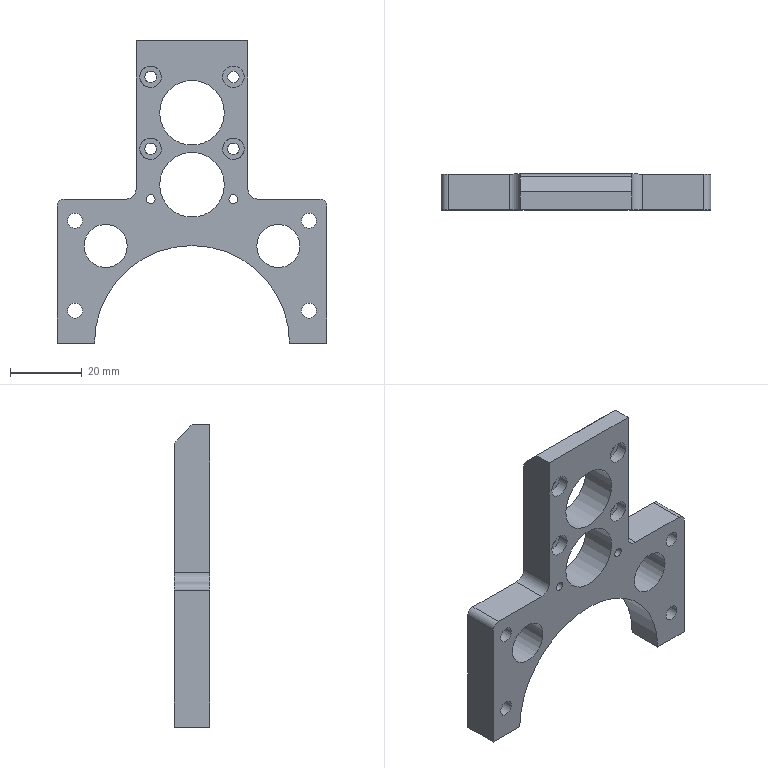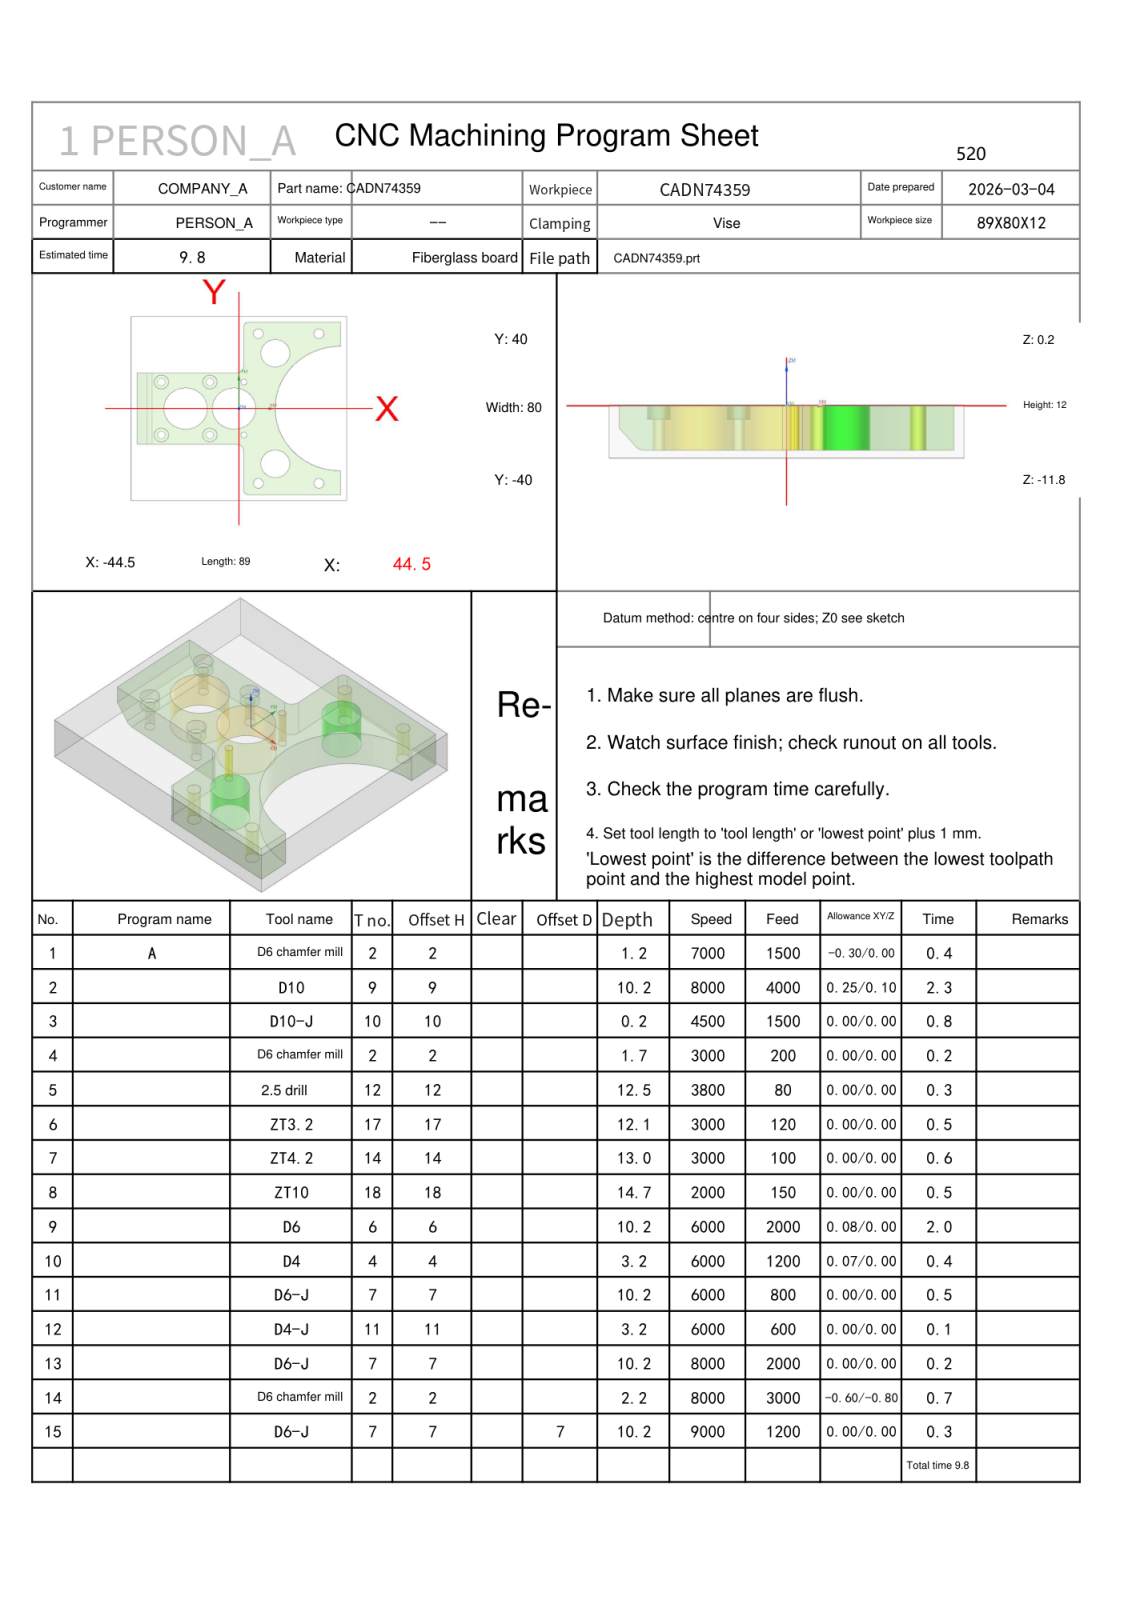NC program | NX | posted by the shop | part box 75 x 10 x 84 mm
Lines 168 to 1025 of 4435:
N2 T09 M06
(D10  D=10. R=0. H=09 ce=0.25 di=0.10)
G00 G90 G54 X55.978 Y-25.62 M03 S8000
G43 H09 Z50.
M08
Z-8.
G01 X55.879 Y-25.636 Z-8.625 F4000.
X55.78 Y-25.652 Z-8.872
X55.682 Y-25.668 Z-9.054
X55.583 Y-25.685 Z-9.2
X55.484 Y-25.701 Z-9.323
X55.386 Y-25.717 Z-9.428
X55.287 Y-25.733 Z-9.52
X55.188 Y-25.749 Z-9.6
X55.089 Y-25.765 Z-9.67
X54.991 Y-25.781 Z-9.732
X54.892 Y-25.798 Z-9.786
X54.793 Y-25.814 Z-9.833
X54.695 Y-25.83 Z-9.874
X54.596 Y-25.846 Z-9.908
X54.497 Y-25.862 Z-9.936
X54.399 Y-25.878 Z-9.96
X54.3 Y-25.894 Z-9.977
X54.201 Y-25.911 Z-9.99
X54.103 Y-25.927 Z-9.997
X54.004 Y-25.943 Z-10.
X51.921 Y-26.284
G03 X51.529 Y-26.606 I.085 J-.503
X51.003 Y-30.391 I13.335 J-3.785
G01 Y-30.428
G03 X50.867 Y-38.753 I808.367 J-17.329
G02 X45.986 Y-45.264 I-7.17 J.29
X39.917 Y-46.285 I-6.261 J18.659
X30.341 Y-46.411 I-9.576 J365.692
X27.499 Y-46.4 I0.0 J365.817
G01 X-42.921 Y-46.382
X-42.933
G02 X-49.794 Y-41.406 I0.0 J7.218
X-50.789 Y-35.332 I19.113 J6.252
X-50.91 Y-25.845 I373.69 J9.487
X-50.9 Y-23.093 I373.811 J0.0
G01 X-50.884 Y38.387
Y38.422
G02 X-45.84 Y45.328 I7.25 J0.0
X-39.701 Y46.297 I6.254 J-19.678
X-30.37 Y46.406 I9.331 J-401.405
X-28.122 Y46.4 I0.0 J-401.514
G01 X42.898 Y46.383
X42.927 Y46.384
G02 X49.811 Y41.386 I0.0 J-7.239
X50.775 Y35.669 I-18.441 J-6.051
X50.912 Y26.372 I-315.381 J-9.297
X50.9 Y23.55 I-315.518 J0.0
G01 X50.877 Y-24.489
G03 X50.286 Y-37.047 I142.408 J-13.003
G02 X45.587 Y-44.06 I-7.974 J.261
X39.258 Y-45.566 I-7.148 J15.994
X30.674 Y-45.811 I-8.584 J150.167
X28.643 Y-45.797 I0.0 J150.412
G01 X-41.507 Y-45.774
G02 X-48.576 Y-41.047 I.213 J7.967
X-50.058 Y-34.839 I15.926 J7.084
X-50.309 Y-26.406 I141.524 J8.433
X-50.297 Y-24.524 I141.775 J0.0
G01 X-50.275 Y36.987
G02 X-45.542 Y44.086 I7.968 J-.186
X-39.152 Y45.576 I7.153 J-16.226
X-30.828 Y45.807 I8.324 J-149.829
X-29.077 Y45.797 I0.0 J-150.06
G01 X41.427 Y45.778
G02 X48.594 Y41.026 I-.134 J-7.982
X50.058 Y34.865 I-15.941 J-7.044
X50.309 Y26.443 I-141.134 J-8.422
X50.297 Y24.551 I-141.385 J0.0
G01 X50.276 Y-23.129
G03 X49.777 Y-33.028 I390.595 J-24.675
G02 X49.784 Y-33.583 I-22.706 J-.555
X49.485 Y-37.255 I-22.713 J0.0
X44.185 Y-43.462 I-8.743 J2.1
X37.719 Y-44.938 I-7.537 J18.117
X28.329 Y-45.215 I-9.389 J158.915
X25.965 Y-45.197 I0.0 J159.192
G01 X-39.955 Y-45.175
G02 X-47.814 Y-39.98 I.188 J8.826
X-49.429 Y-33.31 I17.184 J7.691
X-49.71 Y-24.335 I143.051 J8.974
X-49.696 Y-22.336 I143.332 J0.0
G01 X-49.679 Y35.364
G02 X-44.459 Y43.33 I8.83 J-.092
X-38.022 Y44.911 I7.578 J-16.958
X-28.912 Y45.212 I9.111 J-137.745
X-26.809 Y45.196 I0.0 J-138.046
G01 X39.83 Y45.181
G02 X47.839 Y39.941 I-.065 J-8.84
X49.44 Y33.206 I-17.447 J-7.704
X49.714 Y23.912 I-157.529 J-9.293
X49.697 Y21.632 I-157.803 J0.0
G01 X49.678 Y-21.968
X49.225 Y-31.803
G02 X49.229 Y-32.188 I-20.81 J-.386
X48.802 Y-36.383 I-20.814 J0.0
X45.712 Y-41.212 I-8.978 J2.34
X41.095 Y-43.537 I-7.252 J8.659
X33.371 Y-44.494 I-8.027 J33.122
X22.83 Y-44.603 I-10.541 J509.682
X20.712 Y-44.599 I0.0 J509.791
G01 X-38.488 Y-44.575
G02 X-47.197 Y-38.782 I.085 J9.571
X-48.815 Y-31.864 I18.826 J8.052
X-49.109 Y-22.501 I149.03 J9.363
X-49.095 Y-20.47 I149.324 J0.0
G01 X-49.077 Y33.929
G02 X-43.199 Y42.74 I9.589 J-.031
X-36.212 Y44.33 I8.057 J-19.267
X-26.915 Y44.608 I9.297 J-155.073
X-24.938 Y44.596 I0.0 J-155.351
G01 X38.462 Y44.576
G02 X45.712 Y41.212 I-.038 J-9.578
X47.987 Y36.772 I-8.524 J-7.17
X48.987 Y29.054 I-31.871 J-8.053
X49.103 Y18.823 I-453.561 J-10.231
X49.098 Y16.875 I-453.677 J0.0
G01 X49.081 Y-20.845
G02 X48.512 Y-33.56 I-412.871 J12.098
X47.212 Y-37.787 I-11.192 J1.129
G01 X47.071 Y-38.859
X46.547 Y-40.125
X45.712 Y-41.212
X44.625 Y-42.047
X43.359 Y-42.571
G02 X36.862 Y-43.608 I-18.744 J96.529
X26.221 Y-44.01 I-10.642 J140.772
X24.093 Y-43.994 I0.0 J141.174
G01 X-37.027 Y-43.976
X-37.14 Y-43.977
G02 X-44.43 Y-40.927 I0.0 J10.236
X-47.637 Y-34.44 I9.99 J8.975
X-48.434 Y-25.973 I44.56 J8.467
G01 Y-25.851
G02 X-48.502 Y-16.338 I668.609 J9.513
X-48.498 Y-14.151 I668.677 J0.0
G01 X-48.477 Y32.509
X-48.478 Y32.633
G02 X-45.618 Y39.748 I10.279 J0.0
X-39.076 Y43.109 I9.049 J-9.568
X-30.73 Y43.925 I8.364 J-42.415
X-20.67 Y44.001 I10.06 J-670.02
X-18.79 Y43.998 I0.0 J-670.095
G01 X36.99 Y43.978
G02 X42.15 Y42.73 I-.05 J-11.506
G01 X43.359 Y42.571
X44.625 Y42.047
X45.672 Y41.243
X44.625 Y42.047
X43.359 Y42.571
X38.927 Y43.246
G03 X32.176 Y43.528 I-6.751 J-80.501
X30.655 Y43.514 I0.0 J-80.783
G01 X-27.705 Y43.49
G03 X-28.368 Y43.494 I-.663 J-67.088
X-36.921 Y42.946 I0.0 J-67.091
X-43.506 Y40.512 I1.842 J-15.105
X-47.595 Y33.6 I6.069 J-8.256
X-48.009 Y27.355 I46.897 J-6.245
X-48.002 Y26.539 I47.311 J0.0
G01 X-47.996 Y-22.581
G03 X-48.002 Y-23.52 I71.557 J-.939
X-47.457 Y-32.338 I71.563 J0.0
X-45.059 Y-38.933 I15.291 J1.827
X-38.134 Y-43.088 I8.297 J5.98
X-31.856 Y-43.51 I6.278 J46.515
X-31.013 Y-43.502 I0.0 J46.937
G01 X27.467 Y-43.496
G03 X28.363 Y-43.501 I.897 J84.045
X38.243 Y-42.918 I0.0 J84.049
G01 X39.379 Y-42.75
X41.998
X43.01 Y-42.617
X41.998 Y-42.75
G03 X39.64 Y-42.745 I-2.358 J-552.508
X26.893 Y-42.892 I0.0 J-552.513
G01 X-30.987 Y-42.896
G02 X-31.694 Y-42.903 I-.707 J36.738
X-37.738 Y-42.402 I0.0 J36.745
X-45.639 Y-35.699 I2.086 J10.465
X-47.152 Y-28.384 I22.469 J8.463
X-47.421 Y-19.046 I162.115 J9.338
X-47.415 Y-17.71 I162.384 J0.0
G01 X-47.39 Y26.97
G02 X-47.394 Y27.517 I33.144 J.547
X-46.865 Y33.418 I33.149 J0.0
X-40.255 Y41.119 I10.407 J-2.246
X-32.762 Y42.662 I8.552 J-22.554
X-22.513 Y42.931 I10.25 J-195.098
X-20.047 Y42.916 I0.0 J-195.367
G01 X32.913 Y42.895
G02 X37.059 Y42.75 I-3.312 J-153.901
G01 X42.002
X4.001
G02 X-1.94 Y42.44 I-5.941 J56.745
X-2.948 Y42.449 I0.0 J57.055
G01 X-26.644 Y42.398
G03 X-27.162 Y42.401 I-.518 J-58.199
X-35.911 Y41.739 I0.0 J-58.202
X-42.35 Y39.095 I2.145 J-14.385
X-46.294 Y32.394 I7.049 J-8.66
X-46.907 Y25.431 I39.25 J-6.963
X-46.904 Y24.93 I39.863 J0.0
G01 X-46.964 Y17.118
X-47.071 Y16.859
X-47.25 Y15.502
Y-15.498
G02 X-46.946 Y-20.425 I-41.193 J-5.017
G01 Y-20.474
G03 X-46.475 Y-29.878 I94.099 J0.0
X-44.401 Y-36.66 I17.549 J1.657
X-37.082 Y-41.751 I9.348 J5.635
X-30.309 Y-42.394 I6.773 J35.353
G01 X-30.043 Y-42.393
X-20.803 Y-42.437
X2.063 Y-42.455
X2.387 Y-42.568
X3.999 Y-42.75
X34.179
G02 X34.679 Y-43.25 I0.0 J-.5
X34.447 Y-43.672 I-.5 J0.0
G01 X33.688 Y-44.154
X32.018 Y-45.216 Z-9.9
X31.686 Y-45.427
X31.625 Y-45.46
X31.56 Y-45.484
X31.493 Y-45.499
X31.424 Y-45.505
X4.011 Y-45.829
X3.927 Y-45.823
X3.845 Y-45.802
X3.768 Y-45.769
X3.697 Y-45.723
X3.635 Y-45.666
X3.584 Y-45.599
X3.545 Y-45.524
X3.405 Y-45.195
X2.631 Y-43.374 Z-10.
X2.319 Y-42.658
G03 X1.312 Y-42.24 I-1.103 J-1.237
X-3.973 Y-41.861 I-5.285 J-36.647
X-4.603 Y-41.866 I0.0 J-37.027
G01 X-28.949 Y-41.801
G02 X-29.41 Y-41.804 I-.461 J37.313
X-36.23 Y-41.176 I0.0 J37.315
X-44.694 Y-33.743 I2.238 J11.085
X-46.111 Y-26.101 I25.417 J8.665
G01 X-46.444 Y-18.331
X-47.071 Y-16.859
X-47.142 Y-16.323
X-47.071 Y-16.859
G02 X-46.288 Y-18.758 I-19.509 J-9.157
X-45.837 Y-22.708 I-25.147 J-4.869
G03 X-45.021 Y-30.447 I53.163 J1.699
X-41.905 Y-37.052 I13.689 J2.42
X-35.072 Y-40.683 I8.907 J8.516
X-27.688 Y-41.32 I7.384 J42.526
X-27.309 Y-41.318 I0.0 J43.162
G01 X-4.438 Y-41.397
X-4.27
G02 X.312 Y-41.701 I0.0 J-34.683
G03 X1.817 Y-42.369 I2.752 J4.172
G02 X.115 Y-41.59 I1.508 J5.543
G03 X-3.709 Y-40.929 I-4.076 J-12.18
X-11.989 Y-40.751 I-8.28 J-193.082
X-13.61 Y-40.758 I0.0 J-193.26
G02 X-17.984 Y-40.779 I-4.374 J460.512
X-29.468 Y-40.635 I0.0 J460.533
X-36.376 Y-39.534 I.356 J24.457
X-43.581 Y-32.282 I3.881 J11.062
X-45.006 Y-25.185 I25.784 J8.869
G03 X-45.613 Y-19.657 I-53.321 J-3.05
G01 X-45.772 Y-19.135
X-46.539 Y-18.135
G02 X-45.484 Y-19.685 I-4.89 J-4.462
X-44.673 Y-24.041 I-19.233 J-5.834
G03 X-43.366 Y-31.047 I34.292 J2.772
X-34.429 Y-39.344 I11.592 J3.524
X-26.626 Y-40.207 I7.803 J34.842
G01 X-26.573
G03 X-13.716 Y-40.3 I12.857 J895.985
X-9.973 Y-40.292 I0.0 J896.077
G02 X-8.974 Y-40.284 I.999 J-61.074
X-2.064 Y-40.676 I0.0 J-61.082
X-.642 Y-41.046 I-.299 J-4.06
G03 X.293 Y-41.679 I3.825 J4.643
G02 X-.995 Y-40.8 I12.01 J18.986
G03 X-4.697 Y-39.958 I-4.256 J-10.154
X-13.146 Y-39.669 I-8.449 J-123.288
X-14.816 Y-39.681 I0.0 J-123.577
G02 X-17.977 Y-39.698 I-3.161 J282.289
X-28.411 Y-39.505 I0.0 J282.307
X-35.405 Y-38.215 I.667 J23.218
X-42.507 Y-30.802 I4.436 J11.359
X-43.957 Y-24.497 I29.071 J10.002
G03 X-44.861 Y-20.178 I-22.179 J-2.388
X-45.148 Y-19.645 I-2.368 J-.934
G01 X-45.712 Y-19.212
G02 X-44.343 Y-21.085 I-1.61 J-2.614
X-43.218 Y-26.093 I-38.835 J-11.359
G03 X-40.843 Y-32.734 I19.336 J3.169
X-33.229 Y-38.154 I10.555 J6.769
X-25.263 Y-39.109 I8.099 J33.868
X-10.491 Y-39.236 I15.426 J931.048
G02 X-10.043 Y-39.234 I.448 J-44.89
X-3.185 Y-39.761 I0.0 J-44.892
X-1.326 Y-40.363 I-1.209 J-6.911
G01 X-.647 Y-41.042
G03 X-3.589 Y-39.339 I-3.76 J-3.104
X-10.409 Y-38.673 I-6.821 J-34.624
G01 X-10.487 Y-38.674
X-24.004 Y-38.529
X-24.089
G02 X-32.162 Y-37.667 I0.0 J38.205
X-41.471 Y-29.37 I2.825 J12.541
X-43.15 Y-23.285 I46.847 J16.199
G03 X-44.329 Y-20.212 I-9.432 J-1.856
G02 X-45.101 Y-19.681 I4.994 J8.092
G03 X-44.363 Y-20.162 I1.751 J1.884
G02 X-43.084 Y-22.413 I-3.959 J-3.739
G01 X-41.479 Y-27.725
G03 X-37.233 Y-34.324 I13.721 J4.164
X-29.923 Y-37.464 I9.491 J12.016
X-21.493 Y-38.085 I8.43 J56.981
X-21.014 Y-38.083 I0.0 J57.601
G02 X-20.057 Y-38.081 I.957 J-307.575
X-8.281 Y-38.307 I0.0 J-307.576
X-2.849 Y-39.198 I-.51 J-20.109
X-1.851 Y-39.73 I-.792 J-2.69
G03 X-1.371 Y-40.317 I2.227 J1.328
G02 X-2.031 Y-39.512 I5.118 J4.867
G03 X-5.065 Y-38.243 I-4.075 J-5.479
X-12.566 Y-37.588 I-7.501 J-42.596
G01 X-12.576
G02 X-24.863 Y-37.347 I2.732 J452.627
X-32.465 Y-36.04 I.691 J26.789
X-40.216 Y-28.664 I4.515 J12.505
X-42.261 Y-23.056 I71.553 J29.275
G03 X-43.664 Y-20.469 I-7.417 J-2.347
G01 X-44.43 Y-20.128
G02 X-42.7 Y-21.538 I-.732 J-2.664
X-40.912 Y-25.618 I-21.873 J-12.018
G03 X-37.636 Y-31.607 I18.541 J6.251
X-29.785 Y-36.108 I10.661 J9.499
X-21.143 Y-36.969 I8.645 J42.957
G02 X-9.56 Y-37.254 I-2.044 J-318.823
X-3.802 Y-38.22 I-.712 J-21.872
X-2.276 Y-39.053 I-1.478 J-4.525
G01 X-1.861 Y-39.713
G03 X-4.109 Y-37.8 I-3.368 J-1.68
X-9.824 Y-36.714 I-6.597 J-19.142
X-21.242 Y-36.355 I-13.931 J-261.093
G02 X-29.456 Y-35.443 I.259 J39.8
X-39.091 Y-27.812 I3.147 J13.871
X-41.427 Y-22.807 I236.967 J113.633
G03 X-42.955 Y-20.67 I-6.228 J-2.838
G02 X-43.747 Y-20.41 I2.165 J7.957
G03 X-43.01 Y-20.624 I.982 J2.013
G02 X-41.262 Y-22.523 I-2.552 J-4.103
X-38.894 Y-27.074 I-125.709 J-68.303
G03 X-31.679 Y-33.964 I13.27 J6.674
X-24.1 Y-35.661 I8.982 J22.339
X-13.459 Y-36.056 I13.746 J226.822
G02 X-5.881 Y-36.864 I-.377 J-39.481
X-2.684 Y-38.315 I-1.364 J-7.253
G01 X-2.309 Y-39.001
G02 X-2.739 Y-38.192 I12.18 J7.002
G03 X-5.41 Y-36.612 I-4.104 J-3.887
X-11.976 Y-35.578 I-7.487 J-26.19
G01 X-22.369 Y-35.156
G02 X-30.191 Y-33.719 I1.023 J27.589
X-37.981 Y-27.074 I5.422 J14.245
G03 X-40.656 Y-22.509 I-175.651 J-99.865
X-42.382 Y-20.707 I-4.553 J-2.633
G01 X-43.146 Y-20.599
G02 X-41.045 Y-21.639 I-.022 J-2.687
X-38.39 Y-25.492 I-18.734 J-15.749
G03 X-33.583 Y-31.091 I16.635 J9.42
X-25.612 Y-34.225 I10.381 J14.7
X-17.662 Y-34.86 I9.08 J63.578
G02 X-8.545 Y-35.487 I-1.005 J-81.175
X-3.814 Y-36.968 I-1.501 J-13.094
X-2.814 Y-37.84 I-1.631 J-2.88
G01 X-2.616 Y-38.406
G03 X-4.122 Y-36.503 I-2.823 J-.687
X-9.004 Y-34.935 I-6.496 J-11.843
X-17.219 Y-34.284 I-10.043 J-74.573
G02 X-26.109 Y-33.433 I.894 J56.153
X-36.867 Y-26.432 I3.018 J16.404
G03 X-39.87 Y-22.252 I-72.199 J-48.71
X-41.584 Y-20.772 I-4.585 J-3.578
G01 X-42.418 Y-20.695
G02 X-41.412 Y-20.805 I-.543 J-9.629
X-39.051 Y-22.778 I-2.843 J-5.802
G03 X-35.507 Y-27.29 I132.258 J100.238
X-25.583 Y-32.912 I13.04 J11.448
X-17.297 Y-33.787 I9.867 J53.756
G02 X-8.457 Y-34.608 I-1.687 J-66.153
X-3.82 Y-36.361 I-1.732 J-11.594
X-2.85 Y-37.736 I-1.04 J-1.763
G03 X-4.524 Y-35.6 I-3.188 J-.774
X-9.795 Y-33.889 I-7.052 J-12.752
X-18.439 Y-33.122 I-12.591 J-92.801
G02 X-26.617 Y-31.926 I1.547 J39.13
X-35.67 Y-25.932 I4.989 J17.369
G03 X-39.088 Y-21.977 I-50.57 J-40.249
X-40.876 Y-20.75 I-3.399 J-3.036
G01 X-41.656
G02 X-41.285 Y-20.726 I.371 J-2.903
X-39.363 Y-21.446 I0.0 J-2.926
X-36.797 Y-23.948 I-11.544 J-14.405
G03 X-31.913 Y-28.668 I22.885 J18.795
X-23.036 Y-32.089 I11.602 J16.879
X-14.2 Y-32.928 I15.114 J112.176
G02 X-6.901 Y-34.154 I-1.794 J-33.03
X-3.497 Y-36.09 I-2.113 J-7.674
X-3.067 Y-37.058 I-.874 J-.967
G01 X-3.068 Y-37.113
G03 X-4.062 Y-35.282 I-2.357 J-.094
X-8.461 Y-33.262 I-6.557 J-8.478
X-16.022 Y-32.21 I-10.477 J-47.597
G02 X-24.346 Y-31.142 I3.296 J58.686
X-34.687 Y-25.208 I4.429 J19.695
G03 X-38.432 Y-21.582 I-31.576 J-28.861
X-39.893 Y-20.75 I-3.002 J-3.574
G01 X-40.853
G02 X-40.415 Y-20.725 I.438 J-3.843
X-39.238 Y-20.908 I0.0 J-3.868
X-36.281 Y-23.044 I-4.683 J-9.601
G03 X-31.381 Y-27.349 I33.392 J33.065
X-22.004 Y-31.01 I12.511 J18.205
X-13.429 Y-31.983 I22.048 J155.982
G02 X-6.579 Y-33.457 I-2.306 J-27.379
X-3.445 Y-35.582 I-2.319 J-6.792
X-3.119 Y-36.575 I-1.347 J-.993
G01 X-3.12 Y-36.65
G03 X-4.307 Y-34.396 I-2.819 J-.045
X-8.869 Y-32.271 I-7.049 J-9.178
X-15.358 Y-31.212 I-10.765 J-45.516
G02 X-23.481 Y-30.025 I5.344 J64.977
X-33.651 Y-24.567 I5.286 J22.053
G03 X-37.589 Y-21.323 I-24.981 J-26.311
X-38.763 Y-20.75 I-2.88 J-4.409
G01 X-39.843
G02 X-39.353 Y-20.725 I.49 J-4.802
X-38.112 Y-20.887 I0.0 J-4.827
X-34.867 Y-22.977 I-4.954 J-11.26
G03 X-29.258 Y-27.108 I27.137 J30.963
X-19.872 Y-30.138 I12.68 J23.228
G02 X-11.621 Y-31.251 I-58.085 J-461.973
X-5.525 Y-33.171 I-2.607 J-18.915
X-3.282 Y-35.269 I-2.463 J-4.882
G01 X-3.196 Y-35.976
Y-35.949
G03 X-4.296 Y-33.698 I-2.854 J0.0
X-8.928 Y-31.36 I-7.358 J-8.822
X-15.177 Y-30.175 I-11.588 J-44.028
G02 X-23.207 Y-28.78 I6.811 J63.02
X-32.501 Y-24.02 I6.829 J24.786
G03 X-36.642 Y-21.101 I-20.963 J-25.34
X-37.479 Y-20.75 I-5.556 J-12.064
G01 X-38.739
G02 X-38.18 Y-20.729 I.558 J-7.498
X-36.998 Y-20.823 I0.0 J-7.519
X-33.829 Y-22.531 I-3.792 J-10.825
G03 X-27.914 Y-26.342 I29.727 J39.642
X-18.64 Y-29.16 I13.445 J27.581
G02 X-10.486 Y-30.525 I-17.258 J-128.115
X-4.937 Y-32.783 I-2.934 J-15.157
X-3.254 Y-34.783 I-2.336 J-3.673
G01 X-3.25 Y-35.355
G03 X-3.239 Y-35.115 I-2.637 J.24
X-4.1 Y-33.161 I-2.648 J0.0
X-8.5 Y-30.6 I-7.389 J-7.633
X-15.25 Y-29.099 I-12.561 J-40.567
G02 X-23.455 Y-27.386 I7.507 J56.475
X-31.899 Y-23.091 I10.047 J30.199
G03 X-35.938 Y-20.766 I-12.406 J-16.881
G01 X-37.47 Y-20.75
G02 X-36.842 Y-20.73 I.628 J-10.069
X-35.548 Y-20.814 I0.0 J-10.088
X-32.096 Y-22.482 I-4.136 J-12.961
G03 X-24.942 Y-26.26 I23.464 J35.773
X-16.517 Y-28.384 I14.885 J41.269
G02 X-8.773 Y-30.084 I-7.577 J-53.015
X-4.188 Y-32.664 I-3.225 J-11.093
X-3.25 Y-34.116 I-2.443 J-2.608
G01 Y-34.716
G03 X-3.236 Y-34.435 I-2.808 J.281
X-4.097 Y-32.405 I-2.822 J0.0
X-8.449 Y-29.72 I-7.677 J-7.572
X-15.703 Y-27.939 I-14.452 J-43.196
G02 X-24.539 Y-25.671 I7.513 J47.613
X-31.516 Y-22.116 I18.838 J45.599
G03 X-34.397 Y-20.75 I-8.099 J-13.358
G01 X-36.017
G02 X-35.296 Y-20.726 I.721 J-10.675
X-33.761 Y-20.836 I0.0 J-10.699
X-30.007 Y-22.492 I-5.598 J-17.769
G03 X-16.856 Y-27.203 I20.454 J36.392
G02 X-9.05 Y-29.075 I-10.52 J-61.069
X-4.298 Y-31.774 I-3.607 J-11.883
X-3.25 Y-33.382 I-2.64 J-2.866
G01 Y-34.102
G03 X-3.231 Y-33.758 I-3.114 J.344
X-4.253 Y-31.442 I-3.133 J0.0
X-8.918 Y-28.632 I-8.349 J-8.582
X-15.063 Y-26.984 I-15.34 J-44.908
G02 X-24.376 Y-24.418 I10.392 J55.901
X-30.93 Y-21.372 I44.954 J105.323
G03 X-32.536 Y-20.75 I-9.9 J-23.164
G01 X-34.336
G02 X-33.543 Y-20.727 I.792 J-13.845
X-31.866 Y-20.829 I0.0 J-13.868
X-27.9 Y-22.357 I-6.216 J-22.049
G03 X-16.113 Y-26.247 I22.383 J48.021
G02 X-8.541 Y-28.343 I-9.85 J-50.296
X-4.122 Y-31.158 I-3.937 J-11.057
X-3.25 Y-32.603 I-2.853 J-2.706
G01 Y-33.263
G03 X-3.236 Y-32.962 I-3.17 J.301
X-4.22 Y-30.659 I-3.184 J0.0
X-8.758 Y-27.764 I-8.569 J-8.424
X-15.012 Y-25.911 I-16.544 J-44.374
G02 X-28.515 Y-21.428 I14.357 J65.813
G03 X-30.408 Y-20.75 I-19.495 J-51.474
G01 X-32.448
G02 X-31.539 Y-20.729 I.909 J-19.626
X-29.712 Y-20.814 I0.0 J-19.647
X-25.11 Y-22.359 I-7.543 J-30.094
G03 X-14.104 Y-25.644 I30.506 J82.133
G02 X-7.135 Y-28.076 I-7.239 J-31.941
X-3.587 Y-31.05 I-3.871 J-8.221
X-3.226 Y-32.208 I-1.678 J-1.158
X-3.25 Y-32.518 I-2.039 J0.0
G03 X-3.231 Y-32.167 I-3.25 J.351
X-4.186 Y-29.858 I-3.269 J0.0
X-8.737 Y-26.831 I-8.889 J-8.429
X-14.813 Y-24.876 I-17.578 J-44.204
G02 X-26.67 Y-21.141 I27.128 J106.809
G01 X-27.944 Y-20.75
X-30.284
G02 X-29.232 Y-20.729 I1.053 J-27.038
X-27.152 Y-20.809 I0.0 J-27.059
X-22.341 Y-22.19 I-8.254 J-37.833
G03 X-12.347 Y-25.089 I109.646 J359.286
G02 X-5.897 Y-27.922 I-6.186 J-22.842
X-3.285 Y-30.817 I-3.669 J-5.938
X-3.249 Y-31.593 I-8.562 J-.776
G01 X-3.25 Y-31.691
G03 X-3.231 Y-31.338 I-3.323 J.352
X-4.181 Y-29.005 I-3.341 J0.0
X-8.662 Y-25.912 I-9.178 J-8.503
X-16.534 Y-23.295 I-22.63 J-54.924
G01 X-25.009 Y-20.759
X-27.713 Y-20.75
G02 X-26.519 Y-20.73 I1.194 J-36.754
X-24.112 Y-20.809 I0.0 J-36.774
X-18.998 Y-22.093 I-8.993 J-46.638
X-9.981 Y-24.902 I-26.353 J-100.494
X-4.717 Y-27.984 I-5.494 J-15.419
X-3.25 Y-30.12 I-3.309 J-3.845
G01 Y-30.9
G03 X-3.23 Y-30.527 I-3.519 J.373
X-4.281 Y-28.011 I-3.539 J0.0
X-8.974 Y-24.804 I-9.811 J-9.318
X-17.431 Y-21.929 I-25.406 J-60.859
X-21.758 Y-20.75 I-108.618 J-390.165
G01 X-24.818
G02 X-23.388 Y-20.728 I1.43 J-46.12
X-20.621 Y-20.811 I0.0 J-46.142
X-12.232 Y-23.063 I-9.307 J-51.428
X-5.753 Y-26.211 I-7.095 J-22.842
X-3.277 Y-29.115 I-4.045 J-5.957
G01 X-3.25 Y-30.024
G03 X-3.23 Y-29.648 I-3.548 J.376
X-4.254 Y-27.146 I-3.568 J0.0
X-8.933 Y-23.843 I-10.086 J-9.322
X-18.166 Y-20.75 I-20.561 J-46.046
G01 X-21.346
G02 X-19.836 Y-20.726 I1.51 J-48.359
X-17.017 Y-20.809 I0.0 J-48.383
X-6.617 Y-24.673 I-4.924 J-29.176
X-3.425 Y-27.889 I-4.536 J-7.695
G01 X-3.25 Y-28.354
Y-29.134
G03 X-3.23 Y-28.752 I-3.569 J.382
X-4.218 Y-26.278 I-3.59 J0.0
X-8.972 Y-22.845 I-10.311 J-9.267
X-14.788 Y-20.75 I-13.654 J-28.79
G01 X-17.728
G02 X-16.309 Y-20.725 I1.42 J-41.077
X-13.929 Y-20.794 I0.0 J-41.101
X-4.997 Y-24.984 I-3.205 J-18.451
X-3.25 Y-27.456 I-3.738 J-4.495
G01 Y-28.236
G03 X-3.231 Y-27.859 I-3.661 J.378
X-4.246 Y-25.32 I-3.681 J0.0
X-9.233 Y-21.771 I-10.371 J-9.294
X-12.014 Y-20.75 I-8.573 J-19.053
G01 X-14.474
G02 X-13.36 Y-20.727 I1.114 J-26.479
X-11.257 Y-20.81 I0.0 J-26.502
X-4.08 Y-25.039 I-2.713 J-12.807
X-3.25 Y-26.542 I-3.587 J-2.963
G01 Y-27.382
G03 X-3.228 Y-26.971 I-3.779 J.411
X-4.304 Y-24.321 I-3.802 J0.0
X-9.86 Y-20.75 I-9.16 J-8.144
G01 X-11.78
G02 X-10.941 Y-20.728 I.839 J-15.999
X-9.226 Y-20.82 I0.0 J-16.021
X-3.521 Y-24.958 I-2.262 J-9.119
G01 X-3.25 Y-25.621
Y-26.461
G03 X-3.228 Y-26.053 I-3.772 J.408
X-4.328 Y-23.382 I-3.794 J0.0
X-8.207 Y-20.75 I-6.827 J-5.888
G01 X-9.767
G02 X-9.097 Y-20.732 I.67 J-12.463
X-7.745 Y-20.805 I0.0 J-12.481
X-3.285 Y-24.568 I-1.813 J-6.674
X-3.248 Y-25.331 I-7.876 J-.763
G01 X-3.25 Y-25.503
G03 X-3.229 Y-25.117 I-3.549 J.386
X-4.303 Y-22.565 I-3.57 J0.0
X-6.929 Y-20.75 I-4.739 J-4.052
G01 X-8.189
G02 X-7.63 Y-20.728 I.56 J-6.979
X-6.463 Y-20.826 I0.0 J-7.002
X-3.25 Y-23.873 I-1.527 J-4.827
G01 Y-24.653
G03 X-3.228 Y-24.27 I-3.312 J.383
X-4.438 Y-21.7 I-3.334 J0.0
X-5.95 Y-20.75 I-2.775 J-2.738
G01 X-6.91
G02 X-6.474 Y-20.727 I.436 J-4.16
X-5.473 Y-20.849 I0.0 J-4.182
X-3.25 Y-23.122 I-1.322 J-3.517
G01 Y-23.782
G03 X-3.231 Y-23.459 I-2.794 J.322
X-4.557 Y-21.072 I-2.812 J0.0
X-5.206 Y-20.75 I-1.316 J-1.838
G01 X-5.926
G02 X-5.586 Y-20.726 I.34 J-2.378
X-3.468 Y-21.996 I0.0 J-2.402
X-3.232 Y-22.811 I-1.292 J-.815
X-3.25 Y-23.047 I-1.528 J0.0
G03 X-3.227 Y-22.736 I-2.068 J.311
X-4.663 Y-20.75 I-2.091 J0.0
G01 X-5.203
G02 X-4.933 Y-20.729 I.27 J-1.719
X-3.25 Y-22.029 I0.0 J-1.74
G01 Y-22.389
G03 X-3.233 Y-22.162 I-1.458 J.226
X-4.28 Y-20.75 I-1.476 J0.0
G01 X-4.64
G02 X-4.425 Y-20.73 I.216 J-1.158
X-3.247 Y-21.908 I0.0 J-1.178
G01 X-3.25 Y-21.995
G03 X-3.231 Y-21.793 I-1.068 J.202
X-4.013 Y-20.75 I-1.087 J0.0
G01 X-4.313
X-4.126 Y-20.73
G02 X-3.247 Y-21.609 I0.0 J-.879
G01 X-3.25 Y-21.681
X-3.239 Y-21.543
G03 X-3.677 Y-20.799 I-.851 J0.0
X-3.899 Y-20.752 I-.222 J-.503
X-4.449 Y-21.302 I0.0 J-.55
X-4.347 Y-21.622 I.55 J0.0
X-3.973 Y-21.963 I.651 J.337
G01 X-3.8 Y-21.991
G03 X-3.25 Y-21.441 I0.0 J.55
G01 X-3.248 Y-21.385
G03 X-3.897 Y-20.735 I-.65 J0.0
G01 X-4.035 Y-20.75
G03 X-4.479 Y-21.021 I.003 J-.504
G01 X-4.815 Y-21.674
X-5.72 Y-23.434 Z-9.9
X-6.205 Y-24.377
X-6.236 Y-24.45
X-6.255 Y-24.527
X-6.261 Y-24.606
Y-34.5
X-6.254 Y-34.945
X-6.235 Y-35.391
X-6.202 Y-35.836
X-6.157 Y-36.279
X-6.098 Y-36.721
X-6.027 Y-37.161
X-5.942 Y-37.599
X-5.845 Y-38.034
X-5.736 Y-38.466
X-5.613 Y-38.895
X-5.479 Y-39.32
X-5.41 Y-39.524
X-5.297 Y-39.844
X-5.17 Y-40.159
X-5.031 Y-40.469
X-4.88 Y-40.772
X-4.716 Y-41.07
X-4.541 Y-41.36
X-4.354 Y-41.644
X-4.156 Y-41.919
X-3.947 Y-42.186
X-3.727 Y-42.445
X-3.497 Y-42.695
X-3.257 Y-42.935
X-3.008 Y-43.166
X-2.591 Y-43.537
X-2.347 Y-43.743
X-2.096 Y-43.94
X-1.836 Y-44.125
X-1.568 Y-44.3
X-1.293 Y-44.462
X-1.012 Y-44.613
X-.724 Y-44.752
X-.431 Y-44.878
X-.132 Y-44.992
X.171 Y-45.093
X.477 Y-45.181
X.788 Y-45.255
X1.101 Y-45.317
X1.438 Y-45.376
X2.134 Y-45.489
X2.833 Y-45.589
X3.533 Y-45.673
X4.235 Y-45.743
X4.938 Y-45.798
X5.642 Y-45.838
X6.346 Y-45.863
X34.081 Y-46.571
X34.813 Y-46.583
X35.545 Y-46.58
X36.277 Y-46.563
X37.008 Y-46.532
X37.739 Y-46.486
X38.468 Y-46.426
X39.197 Y-46.353
X39.923 Y-46.265
X40.648 Y-46.162
X41.371 Y-46.046
X42.091 Y-45.916
X42.809 Y-45.771
X45.573 Y-45.187
X45.799 Y-45.133
X46.022 Y-45.065
X46.241 Y-44.985
X46.455 Y-44.893
X46.664 Y-44.788
X46.866 Y-44.672
X47.061 Y-44.545
X47.248 Y-44.407
X47.428 Y-44.258
X47.599 Y-44.1
X47.76 Y-43.932
X47.912 Y-43.755
X48.053 Y-43.57
X49.438 Y-41.643
X49.479 Y-41.576
X49.509 Y-41.503
X49.527 Y-41.427
X49.532 Y-41.349
X49.526 Y-41.271
X49.507 Y-41.194
X49.477 Y-41.122
X49.436 Y-41.055
X49.075 Y-40.563
X47.905 Y-38.967 Z-10.
X47.264 Y-38.083
G02 X47.229 Y-37.713 I1.919 J.37
X47.353 Y-37.027 I1.954 J0.0
G03 X48.235 Y-29.292 I-42.467 J8.756
X48.635 Y-15.53 I-236.08 J13.763
X48.618 Y-12.68 I-236.481 J0.0
G01 X48.592 Y24.8
G03 X48.596 Y25.522 I-62.438 J.722
X48.032 Y33.894 I-62.442 J0.0
X47.25 Y37.08 I-23.657 J-4.119
X47.071 Y38.859 I-10.555 J-.163
G01 X46.547 Y40.125
X47.071 Y38.859
G02 X47.274 Y36.301 I-16.029 J-2.557
X47.273 Y36.101 I-16.232 J0.0
X48.014 Y22.484 I-124.592 J-13.617
X48.008 Y21.225 I-125.334 J0.0
G01 X47.994 Y-19.555
G02 X47.306 Y-33.274 I-165.745 J1.434
G01 X47.25 Y-33.715
X47.226 Y-37.68
X47.225 Y-36.561
G02 X47.296 Y-26.998 I647.744 J0.0
G03 X47.549 Y-13.362 I-367.734 J13.636
X47.538 Y-10.516 I-367.987 J0.0
G01 X47.507 Y23.724
G03 X47.25 Y30.748 I-159.943 J-2.343
G01 Y36.568
Y27.098
G03 X46.933 Y21.617 I47.261 J-5.481
X46.946 Y20.511 I47.578 J0.0
G01 X46.905 Y-19.108
X46.783 Y-25.029
X47.077 Y-25.761
G02 X47.275 Y-27.99 I-12.42 J-2.228
X47.25 Y-28.782 I-12.619 J0.0
G03 X47.275 Y-27.99 I-12.594 J.792
X47.077 Y-25.761 I-12.619 J0.0
G02 X46.498 Y-23.09 I5.884 J2.672
G01 X46.5 Y-22.948
G02 X46.431 Y-14.387 I532.775 J8.561
X46.457 Y-9.112 I532.843 J0.0
G01 X46.486 Y21.915
X46.59 Y24.566
X47.076 Y25.761
X47.123 Y26.118
X47.076 Y25.761
G03 X46.009 Y21.197 I9.76 J-4.689
X45.842 Y12.36 I233.666 J-8.837
X45.858 Y9.671 I233.833 J0.0
G01 X45.861 Y-20.785
Y-20.873
G03 X46.101 Y-23.864 I18.798 J0.0
G02 X46.771 Y-25.012 I-2.951 J-2.494
G03 X46.075 Y-23.848 I-3.296 J-1.182
G02 X45.485 Y-20.462 I9.533 J3.407
X45.357 Y-11.808 I293.648 J8.653
X45.377 Y-8.381 I293.775 J0.0
G01 X45.406 Y16.823
G02 X45.401 Y17.412 I38.789 J.589
X45.812 Y23.042 I38.794 J0.0
G01 X46.016 Y23.779
X46.567 Y24.511
G03 X45.225 Y21.422 I4.091 J-3.613
X44.799 Y14.734 I52.224 J-6.688
X44.803 Y14.066 I52.651 J0.0
G01 X44.795 Y-16.789
G03 X44.79 Y-17.363 I30.585 J-.575
X45.209 Y-22.407 I30.59 J0.0
X45.755 Y-23.431 I1.423 J.102
G01 X46.116 Y-23.911
G03 X45.404 Y-23.099 I-3.796 J-2.611
G02 X44.596 Y-20.255 I6.152 J3.286
X44.294 Y-13.559 I74.061 J6.696
X44.303 Y-12.38 I74.363 J0.0
G01 X44.323 Y13.589
G02 X44.318 Y14.275 I51.456 J.686
X44.774 Y21.11 I51.461 J0.0
X45.384 Y23.09 I5.24 J-.53
G03 X45.971 Y23.718 I-2.675 J3.088
G02 X45.208 Y22.901 I-5.977 J4.821
G03 X44.17 Y19.746 I6.589 J-3.915
X43.716 Y12.18 I62.816 J-7.566